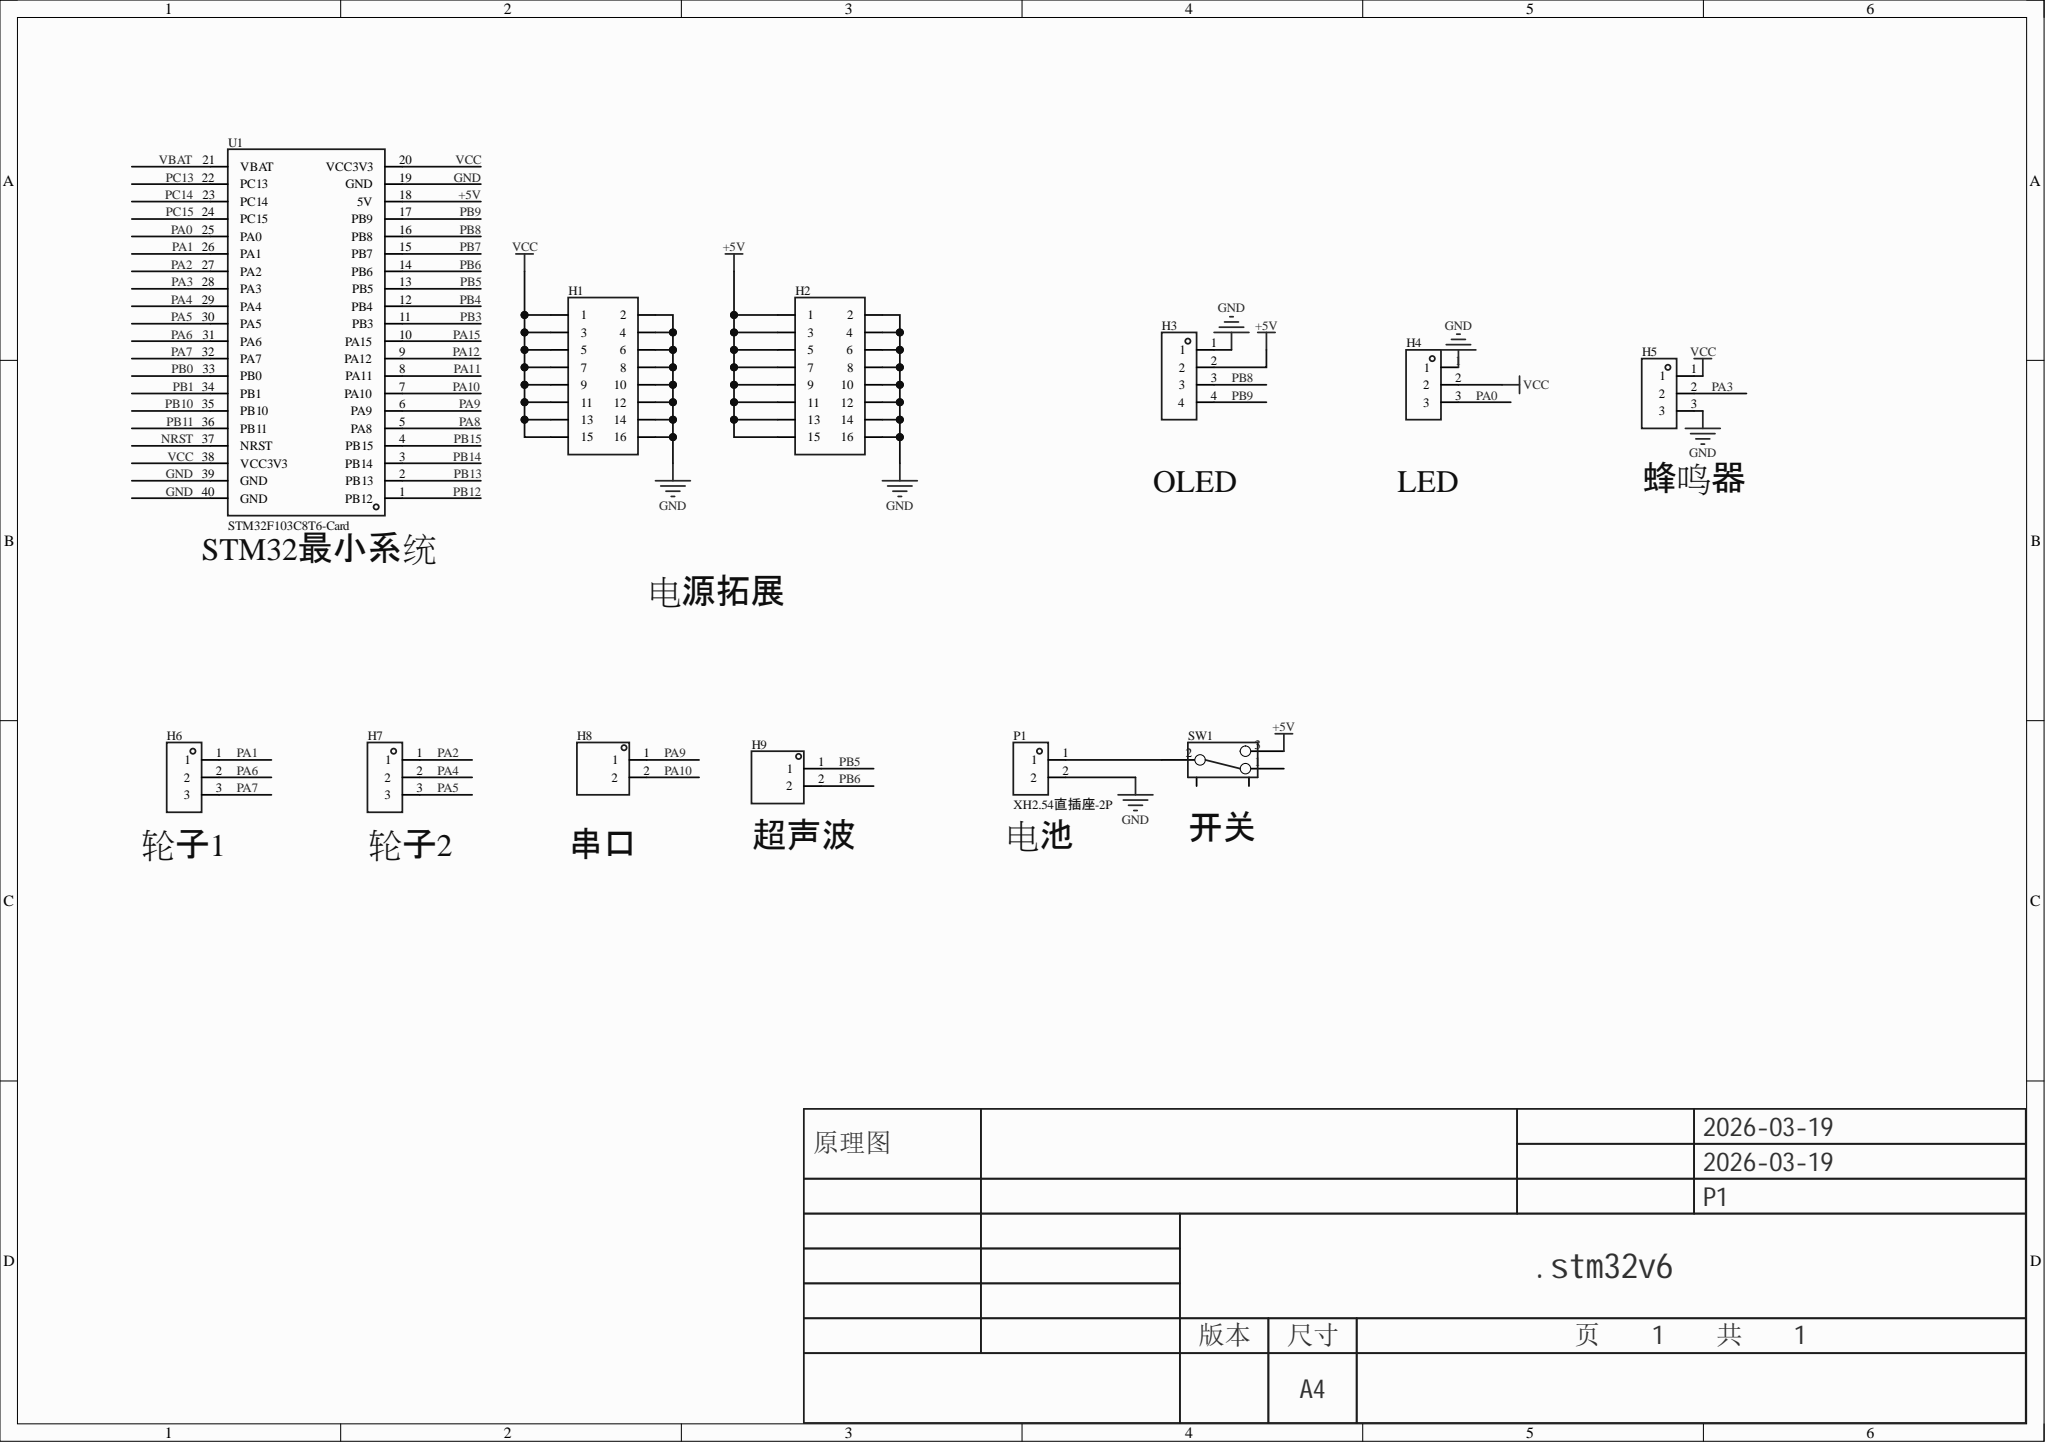Circuit board | Altium Designer | 12 parts | 18 nets
Bill of materials:
Comment,Description,Designator,Footprint,LibRef,Quantity
"","","H1, H2","HDR-TH_16P-P2.54-V-F-R2-C8-S2.54-1","HDR-F_2.54_2x8","2"
"","","H3","HDR-TH_4P-P2.54-V-F","HDR-F_2.54_1x4P","1"
"","","H4, H5, H6, H7","HDR-TH_3P-P2.54-V-F","HDR-F_2.54_1x3P","4"
"","","H8, H9","HDR-TH_2P-P2.54-V-M-1","HDR-M_2.54_1x2P","2"
"XH2.54直插座-2P","","P1","CONN-TH_XH2.54-2P","XH2.54直插座-2P","1"
"","","SW1","拨动开关_侧","拨动开关_侧","1"
"STM32F103C8T6-Card","","U1","CONN-TH_L53.3-W22.9_STM32F103C8T6-CARD","STM32F103C8T6-Card","1"
Netlist (Protel format):
[
H1
HDR-TH_16P-P2.54-V-F-R2-C8-S2.54-1




]
[
H2
HDR-TH_16P-P2.54-V-F-R2-C8-S2.54-1




]
[
H3
HDR-TH_4P-P2.54-V-F




]
[
H4
HDR-TH_3P-P2.54-V-F




]
[
H5
HDR-TH_3P-P2.54-V-F




]
[
H6
HDR-TH_3P-P2.54-V-F




]
[
H7
HDR-TH_3P-P2.54-V-F




]
[
H8
HDR-TH_2P-P2.54-V-M-1




]
[
H9
HDR-TH_2P-P2.54-V-M-1




]
[
P1
CONN-TH_XH2.54-2P
XH2.54直插座-2P



]
[
SW1
拨动开关_侧




]
[
U1
CONN-TH_L53.3-W22.9_STM32F103C8T6-CARD
STM32F103C8T6-Card



]
(
VCC
H1-1
H1-3
H1-5
H1-7
H1-9
H1-11
H1-13
H1-15
H4-2
H5-1
U1-20
U1-38
)
(
PB9
H3-4
U1-17
)
(
PB8
H3-3
U1-16
)
(
PB6
H9-2
U1-14
)
(
PB5
H9-1
U1-13
)
(
PA10
H8-2
U1-7
)
(
PA9
H8-1
U1-6
)
(
PA7
H6-3
U1-32
)
(
PA6
H6-2
U1-31
)
(
PA5
H7-3
U1-30
)
(
PA4
H7-2
U1-29
)
(
PA3
H5-2
U1-28
)
(
PA2
H7-1
U1-27
)
(
PA1
H6-1
U1-26
)
(
PA0
H4-3
U1-25
)
(
NetP1_1
P1-1
SW1-2
)
(
GND
H1-2
H1-4
H1-6
H1-8
H1-10
H1-12
H1-14
H1-16
H2-2
H2-4
H2-6
H2-8
H2-10
H2-12
H2-14
H2-16
H3-1
H4-1
H5-3
P1-2
U1-19
U1-39
U1-40
)
(
+5V
H2-1
H2-3
H2-5
H2-7
H2-9
H2-11
H2-13
H2-15
H3-2
SW1-3
U1-18
)